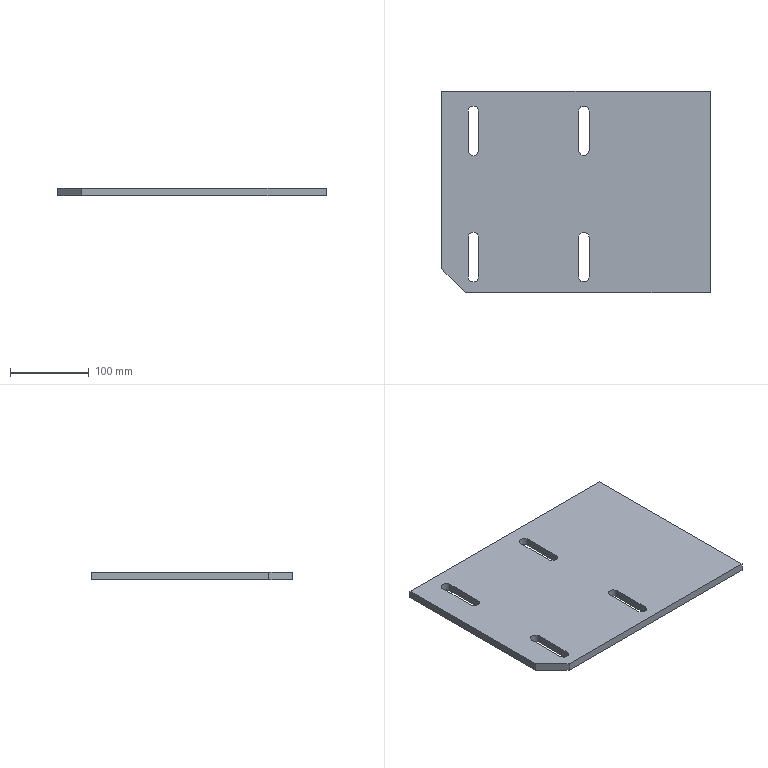Part | SolidWorks | features Extrusion 1 | 1 solid | 23 faces | box 340 x 255 x 10 mm | volume 831191 mm3 | plane 15 | cylinder 8 | commonest cylinder face diameters 13 x8
STEP:
#1=CARTESIAN_POINT('',(0.,-255.,0.));
#2=VERTEX_POINT('',#1);
#3=CARTESIAN_POINT('',(0.,0.,0.));
#4=VERTEX_POINT('',#3);
#5=CARTESIAN_POINT('',(0.,-255.,0.));
#6=DIRECTION('',(0.,1.,0.));
#7=VECTOR('',#6,1000.);
#8=LINE('',#5,#7);
#9=EDGE_CURVE('',#2,#4,#8,.T.);
#10=ORIENTED_EDGE('',*,*,#9,.F.);
#11=CARTESIAN_POINT('',(0.,-255.,-10.));
#12=VERTEX_POINT('',#11);
#13=CARTESIAN_POINT('',(0.,-255.,-10.));
#14=DIRECTION('',(0.,0.,1.));
#15=VECTOR('',#14,1000.);
#16=LINE('',#13,#15);
#17=EDGE_CURVE('',#12,#2,#16,.T.);
#18=ORIENTED_EDGE('',*,*,#17,.F.);
#19=CARTESIAN_POINT('',(0.,0.,-10.));
#20=VERTEX_POINT('',#19);
#21=CARTESIAN_POINT('',(0.,-255.,-10.));
#22=DIRECTION('',(0.,1.,0.));
#23=VECTOR('',#22,1000.);
#24=LINE('',#21,#23);
#25=EDGE_CURVE('',#12,#20,#24,.T.);
#26=ORIENTED_EDGE('',*,*,#25,.T.);
#27=CARTESIAN_POINT('',(0.,0.,-10.));
#28=DIRECTION('',(0.,0.,1.));
#29=VECTOR('',#28,1000.);
#30=LINE('',#27,#29);
#31=EDGE_CURVE('',#20,#4,#30,.T.);
#32=ORIENTED_EDGE('',*,*,#31,.T.);
#33=EDGE_LOOP('',(#10,#18,#26,#32));
#34=FACE_OUTER_BOUND('',#33,.T.);
#35=CARTESIAN_POINT('',(0.,-255.,-10.));
#36=DIRECTION('',(1.,0.,0.));
#37=DIRECTION('',(0.,1.,0.));
#38=AXIS2_PLACEMENT_3D('',#35,#36,#37);
#39=PLANE('',#38);
#40=ADVANCED_FACE('',(#34),#39,.T.);
#41=CARTESIAN_POINT('',(-310.,-255.,0.));
#42=VERTEX_POINT('',#41);
#43=CARTESIAN_POINT('',(-310.,-255.,0.));
#44=DIRECTION('',(1.,0.,0.));
#45=VECTOR('',#44,1000.);
#46=LINE('',#43,#45);
#47=EDGE_CURVE('',#42,#2,#46,.T.);
#48=ORIENTED_EDGE('',*,*,#47,.F.);
#49=CARTESIAN_POINT('',(-310.,-255.,-10.));
#50=VERTEX_POINT('',#49);
#51=CARTESIAN_POINT('',(-310.,-255.,-10.));
#52=DIRECTION('',(0.,0.,1.));
#53=VECTOR('',#52,1000.);
#54=LINE('',#51,#53);
#55=EDGE_CURVE('',#50,#42,#54,.T.);
#56=ORIENTED_EDGE('',*,*,#55,.F.);
#57=CARTESIAN_POINT('',(-310.,-255.,-10.));
#58=DIRECTION('',(1.,0.,0.));
#59=VECTOR('',#58,1000.);
#60=LINE('',#57,#59);
#61=EDGE_CURVE('',#50,#12,#60,.T.);
#62=ORIENTED_EDGE('',*,*,#61,.T.);
#63=ORIENTED_EDGE('',*,*,#17,.T.);
#64=EDGE_LOOP('',(#48,#56,#62,#63));
#65=FACE_OUTER_BOUND('',#64,.T.);
#66=CARTESIAN_POINT('',(-310.,-255.,-10.));
#67=DIRECTION('',(0.,-1.,0.));
#68=DIRECTION('',(0.,0.,-1.));
#69=AXIS2_PLACEMENT_3D('',#66,#67,#68);
#70=PLANE('',#69);
#71=ADVANCED_FACE('',(#65),#70,.T.);
#72=CARTESIAN_POINT('',(-340.,-225.,0.));
#73=VERTEX_POINT('',#72);
#74=CARTESIAN_POINT('',(-340.,-225.,0.));
#75=DIRECTION('',(0.7071,-0.7071,0.));
#76=VECTOR('',#75,1000.);
#77=LINE('',#74,#76);
#78=EDGE_CURVE('',#73,#42,#77,.T.);
#79=ORIENTED_EDGE('',*,*,#78,.F.);
#80=CARTESIAN_POINT('',(-340.,-225.,-10.));
#81=VERTEX_POINT('',#80);
#82=CARTESIAN_POINT('',(-340.,-225.,-10.));
#83=DIRECTION('',(0.,0.,1.));
#84=VECTOR('',#83,1000.);
#85=LINE('',#82,#84);
#86=EDGE_CURVE('',#81,#73,#85,.T.);
#87=ORIENTED_EDGE('',*,*,#86,.F.);
#88=CARTESIAN_POINT('',(-340.,-225.,-10.));
#89=DIRECTION('',(0.7071,-0.7071,0.));
#90=VECTOR('',#89,1000.);
#91=LINE('',#88,#90);
#92=EDGE_CURVE('',#81,#50,#91,.T.);
#93=ORIENTED_EDGE('',*,*,#92,.T.);
#94=ORIENTED_EDGE('',*,*,#55,.T.);
#95=EDGE_LOOP('',(#79,#87,#93,#94));
#96=FACE_OUTER_BOUND('',#95,.T.);
#97=CARTESIAN_POINT('',(-340.,-225.,-10.));
#98=DIRECTION('',(-0.7071,-0.7071,0.));
#99=DIRECTION('',(0.7071,-0.7071,0.));
#100=AXIS2_PLACEMENT_3D('',#97,#98,#99);
#101=PLANE('',#100);
#102=ADVANCED_FACE('',(#96),#101,.T.);
#103=CARTESIAN_POINT('',(-340.,0.,0.));
#104=VERTEX_POINT('',#103);
#105=CARTESIAN_POINT('',(-340.,0.,0.));
#106=DIRECTION('',(0.,-1.,0.));
#107=VECTOR('',#106,1000.);
#108=LINE('',#105,#107);
#109=EDGE_CURVE('',#104,#73,#108,.T.);
#110=ORIENTED_EDGE('',*,*,#109,.F.);
#111=CARTESIAN_POINT('',(-340.,0.,-10.));
#112=VERTEX_POINT('',#111);
#113=CARTESIAN_POINT('',(-340.,0.,-10.));
#114=DIRECTION('',(0.,0.,1.));
#115=VECTOR('',#114,1000.);
#116=LINE('',#113,#115);
#117=EDGE_CURVE('',#112,#104,#116,.T.);
#118=ORIENTED_EDGE('',*,*,#117,.F.);
#119=CARTESIAN_POINT('',(-340.,0.,-10.));
#120=DIRECTION('',(0.,-1.,0.));
#121=VECTOR('',#120,1000.);
#122=LINE('',#119,#121);
#123=EDGE_CURVE('',#112,#81,#122,.T.);
#124=ORIENTED_EDGE('',*,*,#123,.T.);
#125=ORIENTED_EDGE('',*,*,#86,.T.);
#126=EDGE_LOOP('',(#110,#118,#124,#125));
#127=FACE_OUTER_BOUND('',#126,.T.);
#128=CARTESIAN_POINT('',(-340.,0.,-10.));
#129=DIRECTION('',(-1.,0.,0.));
#130=DIRECTION('',(0.,-1.,0.));
#131=AXIS2_PLACEMENT_3D('',#128,#129,#130);
#132=PLANE('',#131);
#133=ADVANCED_FACE('',(#127),#132,.T.);
#134=CARTESIAN_POINT('',(0.,0.,0.));
#135=DIRECTION('',(-1.,0.,0.));
#136=VECTOR('',#135,1000.);
#137=LINE('',#134,#136);
#138=EDGE_CURVE('',#4,#104,#137,.T.);
#139=ORIENTED_EDGE('',*,*,#138,.F.);
#140=ORIENTED_EDGE('',*,*,#31,.F.);
#141=CARTESIAN_POINT('',(0.,0.,-10.));
#142=DIRECTION('',(-1.,0.,0.));
#143=VECTOR('',#142,1000.);
#144=LINE('',#141,#143);
#145=EDGE_CURVE('',#20,#112,#144,.T.);
#146=ORIENTED_EDGE('',*,*,#145,.T.);
#147=ORIENTED_EDGE('',*,*,#117,.T.);
#148=EDGE_LOOP('',(#139,#140,#146,#147));
#149=FACE_OUTER_BOUND('',#148,.T.);
#150=CARTESIAN_POINT('',(0.,0.,-10.));
#151=DIRECTION('',(0.,1.,0.));
#152=DIRECTION('',(-1.,0.,0.));
#153=AXIS2_PLACEMENT_3D('',#150,#151,#152);
#154=PLANE('',#153);
#155=ADVANCED_FACE('',(#149),#154,.T.);
#156=CARTESIAN_POINT('',(-153.5,-235.,-10.));
#157=VERTEX_POINT('',#156);
#158=CARTESIAN_POINT('',(-153.5,-185.,-10.));
#159=VERTEX_POINT('',#158);
#160=CARTESIAN_POINT('',(-153.5,-185.,-10.));
#161=DIRECTION('',(0.,1.,0.));
#162=VECTOR('',#161,1000.);
#163=LINE('',#160,#162);
#164=EDGE_CURVE('',#157,#159,#163,.T.);
#165=ORIENTED_EDGE('',*,*,#164,.T.);
#166=CARTESIAN_POINT('',(-166.5,-185.,-10.));
#167=VERTEX_POINT('',#166);
#168=CARTESIAN_POINT('',(-160.,-185.,-10.));
#169=DIRECTION('',(0.,0.,1.));
#170=DIRECTION('',(1.,0.,0.));
#171=AXIS2_PLACEMENT_3D('',#168,#169,#170);
#172=CIRCLE('',#171,6.5);
#173=EDGE_CURVE('',#159,#167,#172,.T.);
#174=ORIENTED_EDGE('',*,*,#173,.T.);
#175=CARTESIAN_POINT('',(-166.5,-235.,-10.));
#176=VERTEX_POINT('',#175);
#177=CARTESIAN_POINT('',(-166.5,-185.,-10.));
#178=DIRECTION('',(0.,-1.,0.));
#179=VECTOR('',#178,1000.);
#180=LINE('',#177,#179);
#181=EDGE_CURVE('',#167,#176,#180,.T.);
#182=ORIENTED_EDGE('',*,*,#181,.T.);
#183=CARTESIAN_POINT('',(-160.,-235.,-10.));
#184=DIRECTION('',(0.,0.,1.));
#185=DIRECTION('',(1.,0.,0.));
#186=AXIS2_PLACEMENT_3D('',#183,#184,#185);
#187=CIRCLE('',#186,6.5);
#188=EDGE_CURVE('',#176,#157,#187,.T.);
#189=ORIENTED_EDGE('',*,*,#188,.T.);
#190=EDGE_LOOP('',(#165,#174,#182,#189));
#191=FACE_BOUND('',#190,.T.);
#192=CARTESIAN_POINT('',(-293.5,-235.,-10.));
#193=VERTEX_POINT('',#192);
#194=CARTESIAN_POINT('',(-293.5,-185.,-10.));
#195=VERTEX_POINT('',#194);
#196=CARTESIAN_POINT('',(-293.5,-185.,-10.));
#197=DIRECTION('',(0.,1.,0.));
#198=VECTOR('',#197,1000.);
#199=LINE('',#196,#198);
#200=EDGE_CURVE('',#193,#195,#199,.T.);
#201=ORIENTED_EDGE('',*,*,#200,.T.);
#202=CARTESIAN_POINT('',(-306.5,-185.,-10.));
#203=VERTEX_POINT('',#202);
#204=CARTESIAN_POINT('',(-300.,-185.,-10.));
#205=DIRECTION('',(0.,0.,1.));
#206=DIRECTION('',(1.,0.,0.));
#207=AXIS2_PLACEMENT_3D('',#204,#205,#206);
#208=CIRCLE('',#207,6.5);
#209=EDGE_CURVE('',#195,#203,#208,.T.);
#210=ORIENTED_EDGE('',*,*,#209,.T.);
#211=CARTESIAN_POINT('',(-306.5,-235.,-10.));
#212=VERTEX_POINT('',#211);
#213=CARTESIAN_POINT('',(-306.5,-185.,-10.));
#214=DIRECTION('',(0.,-1.,0.));
#215=VECTOR('',#214,1000.);
#216=LINE('',#213,#215);
#217=EDGE_CURVE('',#203,#212,#216,.T.);
#218=ORIENTED_EDGE('',*,*,#217,.T.);
#219=CARTESIAN_POINT('',(-300.,-235.,-10.));
#220=DIRECTION('',(0.,0.,1.));
#221=DIRECTION('',(1.,0.,0.));
#222=AXIS2_PLACEMENT_3D('',#219,#220,#221);
#223=CIRCLE('',#222,6.5);
#224=EDGE_CURVE('',#212,#193,#223,.T.);
#225=ORIENTED_EDGE('',*,*,#224,.T.);
#226=EDGE_LOOP('',(#201,#210,#218,#225));
#227=FACE_BOUND('',#226,.T.);
#228=CARTESIAN_POINT('',(-153.5,-75.,-10.));
#229=VERTEX_POINT('',#228);
#230=CARTESIAN_POINT('',(-153.5,-25.,-10.));
#231=VERTEX_POINT('',#230);
#232=CARTESIAN_POINT('',(-153.5,-25.,-10.));
#233=DIRECTION('',(0.,1.,0.));
#234=VECTOR('',#233,1000.);
#235=LINE('',#232,#234);
#236=EDGE_CURVE('',#229,#231,#235,.T.);
#237=ORIENTED_EDGE('',*,*,#236,.T.);
#238=CARTESIAN_POINT('',(-166.5,-25.,-10.));
#239=VERTEX_POINT('',#238);
#240=CARTESIAN_POINT('',(-160.,-25.,-10.));
#241=DIRECTION('',(0.,0.,1.));
#242=DIRECTION('',(1.,0.,0.));
#243=AXIS2_PLACEMENT_3D('',#240,#241,#242);
#244=CIRCLE('',#243,6.5);
#245=EDGE_CURVE('',#231,#239,#244,.T.);
#246=ORIENTED_EDGE('',*,*,#245,.T.);
#247=CARTESIAN_POINT('',(-166.5,-75.,-10.));
#248=VERTEX_POINT('',#247);
#249=CARTESIAN_POINT('',(-166.5,-25.,-10.));
#250=DIRECTION('',(0.,-1.,0.));
#251=VECTOR('',#250,1000.);
#252=LINE('',#249,#251);
#253=EDGE_CURVE('',#239,#248,#252,.T.);
#254=ORIENTED_EDGE('',*,*,#253,.T.);
#255=CARTESIAN_POINT('',(-160.,-75.,-10.));
#256=DIRECTION('',(0.,0.,1.));
#257=DIRECTION('',(1.,0.,0.));
#258=AXIS2_PLACEMENT_3D('',#255,#256,#257);
#259=CIRCLE('',#258,6.5);
#260=EDGE_CURVE('',#248,#229,#259,.T.);
#261=ORIENTED_EDGE('',*,*,#260,.T.);
#262=EDGE_LOOP('',(#237,#246,#254,#261));
#263=FACE_BOUND('',#262,.T.);
#264=CARTESIAN_POINT('',(-293.5,-75.,-10.));
#265=VERTEX_POINT('',#264);
#266=CARTESIAN_POINT('',(-293.5,-25.,-10.));
#267=VERTEX_POINT('',#266);
#268=CARTESIAN_POINT('',(-293.5,-25.,-10.));
#269=DIRECTION('',(0.,1.,0.));
#270=VECTOR('',#269,1000.);
#271=LINE('',#268,#270);
#272=EDGE_CURVE('',#265,#267,#271,.T.);
#273=ORIENTED_EDGE('',*,*,#272,.T.);
#274=CARTESIAN_POINT('',(-306.5,-25.,-10.));
#275=VERTEX_POINT('',#274);
#276=CARTESIAN_POINT('',(-300.,-25.,-10.));
#277=DIRECTION('',(0.,0.,1.));
#278=DIRECTION('',(1.,0.,0.));
#279=AXIS2_PLACEMENT_3D('',#276,#277,#278);
#280=CIRCLE('',#279,6.5);
#281=EDGE_CURVE('',#267,#275,#280,.T.);
#282=ORIENTED_EDGE('',*,*,#281,.T.);
#283=CARTESIAN_POINT('',(-306.5,-75.,-10.));
#284=VERTEX_POINT('',#283);
#285=CARTESIAN_POINT('',(-306.5,-25.,-10.));
#286=DIRECTION('',(0.,-1.,0.));
#287=VECTOR('',#286,1000.);
#288=LINE('',#285,#287);
#289=EDGE_CURVE('',#275,#284,#288,.T.);
#290=ORIENTED_EDGE('',*,*,#289,.T.);
#291=CARTESIAN_POINT('',(-300.,-75.,-10.));
#292=DIRECTION('',(0.,0.,1.));
#293=DIRECTION('',(1.,0.,0.));
#294=AXIS2_PLACEMENT_3D('',#291,#292,#293);
#295=CIRCLE('',#294,6.5);
#296=EDGE_CURVE('',#284,#265,#295,.T.);
#297=ORIENTED_EDGE('',*,*,#296,.T.);
#298=EDGE_LOOP('',(#273,#282,#290,#297));
#299=FACE_BOUND('',#298,.T.);
#300=ORIENTED_EDGE('',*,*,#25,.F.);
#301=ORIENTED_EDGE('',*,*,#61,.F.);
#302=ORIENTED_EDGE('',*,*,#92,.F.);
#303=ORIENTED_EDGE('',*,*,#123,.F.);
#304=ORIENTED_EDGE('',*,*,#145,.F.);
#305=EDGE_LOOP('',(#300,#301,#302,#303,#304));
#306=FACE_OUTER_BOUND('',#305,.T.);
#307=CARTESIAN_POINT('',(0.,0.,-10.));
#308=DIRECTION('',(0.,0.,1.));
#309=DIRECTION('',(1.,0.,0.));
#310=AXIS2_PLACEMENT_3D('',#307,#308,#309);
#311=PLANE('',#310);
#312=ADVANCED_FACE('',(#191,#227,#263,#299,#306),#311,.F.);
#313=CARTESIAN_POINT('',(-153.5,-185.,0.));
#314=VERTEX_POINT('',#313);
#315=CARTESIAN_POINT('',(-166.5,-185.,0.));
#316=VERTEX_POINT('',#315);
#317=CARTESIAN_POINT('',(-160.,-185.,0.));
#318=DIRECTION('',(0.,0.,1.));
#319=DIRECTION('',(1.,0.,0.));
#320=AXIS2_PLACEMENT_3D('',#317,#318,#319);
#321=CIRCLE('',#320,6.5);
#322=EDGE_CURVE('',#314,#316,#321,.T.);
#323=ORIENTED_EDGE('',*,*,#322,.F.);
#324=CARTESIAN_POINT('',(-153.5,-235.,0.));
#325=VERTEX_POINT('',#324);
#326=CARTESIAN_POINT('',(-153.5,-185.,0.));
#327=DIRECTION('',(0.,1.,0.));
#328=VECTOR('',#327,1000.);
#329=LINE('',#326,#328);
#330=EDGE_CURVE('',#325,#314,#329,.T.);
#331=ORIENTED_EDGE('',*,*,#330,.F.);
#332=CARTESIAN_POINT('',(-166.5,-235.,0.));
#333=VERTEX_POINT('',#332);
#334=CARTESIAN_POINT('',(-160.,-235.,0.));
#335=DIRECTION('',(0.,0.,1.));
#336=DIRECTION('',(1.,0.,0.));
#337=AXIS2_PLACEMENT_3D('',#334,#335,#336);
#338=CIRCLE('',#337,6.5);
#339=EDGE_CURVE('',#333,#325,#338,.T.);
#340=ORIENTED_EDGE('',*,*,#339,.F.);
#341=CARTESIAN_POINT('',(-166.5,-185.,0.));
#342=DIRECTION('',(0.,-1.,0.));
#343=VECTOR('',#342,1000.);
#344=LINE('',#341,#343);
#345=EDGE_CURVE('',#316,#333,#344,.T.);
#346=ORIENTED_EDGE('',*,*,#345,.F.);
#347=EDGE_LOOP('',(#323,#331,#340,#346));
#348=FACE_BOUND('',#347,.T.);
#349=CARTESIAN_POINT('',(-293.5,-185.,0.));
#350=VERTEX_POINT('',#349);
#351=CARTESIAN_POINT('',(-306.5,-185.,0.));
#352=VERTEX_POINT('',#351);
#353=CARTESIAN_POINT('',(-300.,-185.,0.));
#354=DIRECTION('',(0.,0.,1.));
#355=DIRECTION('',(1.,0.,0.));
#356=AXIS2_PLACEMENT_3D('',#353,#354,#355);
#357=CIRCLE('',#356,6.5);
#358=EDGE_CURVE('',#350,#352,#357,.T.);
#359=ORIENTED_EDGE('',*,*,#358,.F.);
#360=CARTESIAN_POINT('',(-293.5,-235.,0.));
#361=VERTEX_POINT('',#360);
#362=CARTESIAN_POINT('',(-293.5,-185.,0.));
#363=DIRECTION('',(0.,1.,0.));
#364=VECTOR('',#363,1000.);
#365=LINE('',#362,#364);
#366=EDGE_CURVE('',#361,#350,#365,.T.);
#367=ORIENTED_EDGE('',*,*,#366,.F.);
#368=CARTESIAN_POINT('',(-306.5,-235.,0.));
#369=VERTEX_POINT('',#368);
#370=CARTESIAN_POINT('',(-300.,-235.,0.));
#371=DIRECTION('',(0.,0.,1.));
#372=DIRECTION('',(1.,0.,0.));
#373=AXIS2_PLACEMENT_3D('',#370,#371,#372);
#374=CIRCLE('',#373,6.5);
#375=EDGE_CURVE('',#369,#361,#374,.T.);
#376=ORIENTED_EDGE('',*,*,#375,.F.);
#377=CARTESIAN_POINT('',(-306.5,-185.,0.));
#378=DIRECTION('',(0.,-1.,0.));
#379=VECTOR('',#378,1000.);
#380=LINE('',#377,#379);
#381=EDGE_CURVE('',#352,#369,#380,.T.);
#382=ORIENTED_EDGE('',*,*,#381,.F.);
#383=EDGE_LOOP('',(#359,#367,#376,#382));
#384=FACE_BOUND('',#383,.T.);
#385=CARTESIAN_POINT('',(-153.5,-25.,0.));
#386=VERTEX_POINT('',#385);
#387=CARTESIAN_POINT('',(-166.5,-25.,0.));
#388=VERTEX_POINT('',#387);
#389=CARTESIAN_POINT('',(-160.,-25.,0.));
#390=DIRECTION('',(0.,0.,1.));
#391=DIRECTION('',(1.,0.,0.));
#392=AXIS2_PLACEMENT_3D('',#389,#390,#391);
#393=CIRCLE('',#392,6.5);
#394=EDGE_CURVE('',#386,#388,#393,.T.);
#395=ORIENTED_EDGE('',*,*,#394,.F.);
#396=CARTESIAN_POINT('',(-153.5,-75.,0.));
#397=VERTEX_POINT('',#396);
#398=CARTESIAN_POINT('',(-153.5,-25.,0.));
#399=DIRECTION('',(0.,1.,0.));
#400=VECTOR('',#399,1000.);
#401=LINE('',#398,#400);
#402=EDGE_CURVE('',#397,#386,#401,.T.);
#403=ORIENTED_EDGE('',*,*,#402,.F.);
#404=CARTESIAN_POINT('',(-166.5,-75.,0.));
#405=VERTEX_POINT('',#404);
#406=CARTESIAN_POINT('',(-160.,-75.,0.));
#407=DIRECTION('',(0.,0.,1.));
#408=DIRECTION('',(1.,0.,0.));
#409=AXIS2_PLACEMENT_3D('',#406,#407,#408);
#410=CIRCLE('',#409,6.5);
#411=EDGE_CURVE('',#405,#397,#410,.T.);
#412=ORIENTED_EDGE('',*,*,#411,.F.);
#413=CARTESIAN_POINT('',(-166.5,-25.,0.));
#414=DIRECTION('',(0.,-1.,0.));
#415=VECTOR('',#414,1000.);
#416=LINE('',#413,#415);
#417=EDGE_CURVE('',#388,#405,#416,.T.);
#418=ORIENTED_EDGE('',*,*,#417,.F.);
#419=EDGE_LOOP('',(#395,#403,#412,#418));
#420=FACE_BOUND('',#419,.T.);
#421=CARTESIAN_POINT('',(-293.5,-25.,0.));
#422=VERTEX_POINT('',#421);
#423=CARTESIAN_POINT('',(-306.5,-25.,0.));
#424=VERTEX_POINT('',#423);
#425=CARTESIAN_POINT('',(-300.,-25.,0.));
#426=DIRECTION('',(0.,0.,1.));
#427=DIRECTION('',(1.,0.,0.));
#428=AXIS2_PLACEMENT_3D('',#425,#426,#427);
#429=CIRCLE('',#428,6.5);
#430=EDGE_CURVE('',#422,#424,#429,.T.);
#431=ORIENTED_EDGE('',*,*,#430,.F.);
#432=CARTESIAN_POINT('',(-293.5,-75.,0.));
#433=VERTEX_POINT('',#432);
#434=CARTESIAN_POINT('',(-293.5,-25.,0.));
#435=DIRECTION('',(0.,1.,0.));
#436=VECTOR('',#435,1000.);
#437=LINE('',#434,#436);
#438=EDGE_CURVE('',#433,#422,#437,.T.);
#439=ORIENTED_EDGE('',*,*,#438,.F.);
#440=CARTESIAN_POINT('',(-306.5,-75.,0.));
#441=VERTEX_POINT('',#440);
#442=CARTESIAN_POINT('',(-300.,-75.,0.));
#443=DIRECTION('',(0.,0.,1.));
#444=DIRECTION('',(1.,0.,0.));
#445=AXIS2_PLACEMENT_3D('',#442,#443,#444);
#446=CIRCLE('',#445,6.5);
#447=EDGE_CURVE('',#441,#433,#446,.T.);
#448=ORIENTED_EDGE('',*,*,#447,.F.);
#449=CARTESIAN_POINT('',(-306.5,-25.,0.));
#450=DIRECTION('',(0.,-1.,0.));
#451=VECTOR('',#450,1000.);
#452=LINE('',#449,#451);
#453=EDGE_CURVE('',#424,#441,#452,.T.);
#454=ORIENTED_EDGE('',*,*,#453,.F.);
#455=EDGE_LOOP('',(#431,#439,#448,#454));
#456=FACE_BOUND('',#455,.T.);
#457=ORIENTED_EDGE('',*,*,#9,.T.);
#458=ORIENTED_EDGE('',*,*,#138,.T.);
#459=ORIENTED_EDGE('',*,*,#109,.T.);
#460=ORIENTED_EDGE('',*,*,#78,.T.);
#461=ORIENTED_EDGE('',*,*,#47,.T.);
#462=EDGE_LOOP('',(#457,#458,#459,#460,#461));
#463=FACE_OUTER_BOUND('',#462,.T.);
#464=CARTESIAN_POINT('',(0.,0.,0.));
#465=DIRECTION('',(0.,0.,1.));
#466=DIRECTION('',(1.,0.,0.));
#467=AXIS2_PLACEMENT_3D('',#464,#465,#466);
#468=PLANE('',#467);
#469=ADVANCED_FACE('',(#348,#384,#420,#456,#463),#468,.T.);
#470=ORIENTED_EDGE('',*,*,#430,.T.);
#471=CARTESIAN_POINT('',(-306.5,-25.,-10.));
#472=DIRECTION('',(0.,0.,1.));
#473=VECTOR('',#472,1000.);
#474=LINE('',#471,#473);
#475=EDGE_CURVE('',#275,#424,#474,.T.);
#476=ORIENTED_EDGE('',*,*,#475,.F.);
#477=ORIENTED_EDGE('',*,*,#281,.F.);
#478=CARTESIAN_POINT('',(-293.5,-25.,-10.));
#479=DIRECTION('',(0.,0.,1.));
#480=VECTOR('',#479,1000.);
#481=LINE('',#478,#480);
#482=EDGE_CURVE('',#267,#422,#481,.T.);
#483=ORIENTED_EDGE('',*,*,#482,.T.);
#484=EDGE_LOOP('',(#470,#476,#477,#483));
#485=FACE_OUTER_BOUND('',#484,.T.);
#486=CARTESIAN_POINT('',(-300.,-25.,-10.));
#487=DIRECTION('',(0.,0.,1.));
#488=DIRECTION('',(1.,0.,0.));
#489=AXIS2_PLACEMENT_3D('',#486,#487,#488);
#490=CYLINDRICAL_SURFACE('',#489,6.5);
#491=ADVANCED_FACE('',(#485),#490,.F.);
#492=ORIENTED_EDGE('',*,*,#438,.T.);
#493=ORIENTED_EDGE('',*,*,#482,.F.);
#494=ORIENTED_EDGE('',*,*,#272,.F.);
#495=CARTESIAN_POINT('',(-293.5,-75.,-10.));
#496=DIRECTION('',(0.,0.,1.));
#497=VECTOR('',#496,1000.);
#498=LINE('',#495,#497);
#499=EDGE_CURVE('',#265,#433,#498,.T.);
#500=ORIENTED_EDGE('',*,*,#499,.T.);
#501=EDGE_LOOP('',(#492,#493,#494,#500));
#502=FACE_OUTER_BOUND('',#501,.T.);
#503=CARTESIAN_POINT('',(-293.5,-25.,-10.));
#504=DIRECTION('',(1.,0.,0.));
#505=DIRECTION('',(0.,0.,-1.));
#506=AXIS2_PLACEMENT_3D('',#503,#504,#505);
#507=PLANE('',#506);
#508=ADVANCED_FACE('',(#502),#507,.F.);
#509=ORIENTED_EDGE('',*,*,#447,.T.);
#510=ORIENTED_EDGE('',*,*,#499,.F.);
#511=ORIENTED_EDGE('',*,*,#296,.F.);
#512=CARTESIAN_POINT('',(-306.5,-75.,-10.));
#513=DIRECTION('',(0.,0.,1.));
#514=VECTOR('',#513,1000.);
#515=LINE('',#512,#514);
#516=EDGE_CURVE('',#284,#441,#515,.T.);
#517=ORIENTED_EDGE('',*,*,#516,.T.);
#518=EDGE_LOOP('',(#509,#510,#511,#517));
#519=FACE_OUTER_BOUND('',#518,.T.);
#520=CARTESIAN_POINT('',(-300.,-75.,-10.));
#521=DIRECTION('',(0.,0.,1.));
#522=DIRECTION('',(1.,0.,0.));
#523=AXIS2_PLACEMENT_3D('',#520,#521,#522);
#524=CYLINDRICAL_SURFACE('',#523,6.5);
#525=ADVANCED_FACE('',(#519),#524,.F.);
#526=ORIENTED_EDGE('',*,*,#453,.T.);
#527=ORIENTED_EDGE('',*,*,#516,.F.);
#528=ORIENTED_EDGE('',*,*,#289,.F.);
#529=ORIENTED_EDGE('',*,*,#475,.T.);
#530=EDGE_LOOP('',(#526,#527,#528,#529));
#531=FACE_OUTER_BOUND('',#530,.T.);
#532=CARTESIAN_POINT('',(-306.5,-25.,-10.));
#533=DIRECTION('',(-1.,0.,0.));
#534=DIRECTION('',(0.,0.,1.));
#535=AXIS2_PLACEMENT_3D('',#532,#533,#534);
#536=PLANE('',#535);
#537=ADVANCED_FACE('',(#531),#536,.F.);
#538=ORIENTED_EDGE('',*,*,#394,.T.);
#539=CARTESIAN_POINT('',(-166.5,-25.,-10.));
#540=DIRECTION('',(0.,0.,1.));
#541=VECTOR('',#540,1000.);
#542=LINE('',#539,#541);
#543=EDGE_CURVE('',#239,#388,#542,.T.);
#544=ORIENTED_EDGE('',*,*,#543,.F.);
#545=ORIENTED_EDGE('',*,*,#245,.F.);
#546=CARTESIAN_POINT('',(-153.5,-25.,-10.));
#547=DIRECTION('',(0.,0.,1.));
#548=VECTOR('',#547,1000.);
#549=LINE('',#546,#548);
#550=EDGE_CURVE('',#231,#386,#549,.T.);
#551=ORIENTED_EDGE('',*,*,#550,.T.);
#552=EDGE_LOOP('',(#538,#544,#545,#551));
#553=FACE_OUTER_BOUND('',#552,.T.);
#554=CARTESIAN_POINT('',(-160.,-25.,-10.));
#555=DIRECTION('',(0.,0.,1.));
#556=DIRECTION('',(1.,0.,0.));
#557=AXIS2_PLACEMENT_3D('',#554,#555,#556);
#558=CYLINDRICAL_SURFACE('',#557,6.5);
#559=ADVANCED_FACE('',(#553),#558,.F.);
#560=ORIENTED_EDGE('',*,*,#402,.T.);
#561=ORIENTED_EDGE('',*,*,#550,.F.);
#562=ORIENTED_EDGE('',*,*,#236,.F.);
#563=CARTESIAN_POINT('',(-153.5,-75.,-10.));
#564=DIRECTION('',(0.,0.,1.));
#565=VECTOR('',#564,1000.);
#566=LINE('',#563,#565);
#567=EDGE_CURVE('',#229,#397,#566,.T.);
#568=ORIENTED_EDGE('',*,*,#567,.T.);
#569=EDGE_LOOP('',(#560,#561,#562,#568));
#570=FACE_OUTER_BOUND('',#569,.T.);
#571=CARTESIAN_POINT('',(-153.5,-25.,-10.));
#572=DIRECTION('',(1.,0.,0.));
#573=DIRECTION('',(0.,0.,-1.));
#574=AXIS2_PLACEMENT_3D('',#571,#572,#573);
#575=PLANE('',#574);
#576=ADVANCED_FACE('',(#570),#575,.F.);
#577=ORIENTED_EDGE('',*,*,#411,.T.);
#578=ORIENTED_EDGE('',*,*,#567,.F.);
#579=ORIENTED_EDGE('',*,*,#260,.F.);
#580=CARTESIAN_POINT('',(-166.5,-75.,-10.));
#581=DIRECTION('',(0.,0.,1.));
#582=VECTOR('',#581,1000.);
#583=LINE('',#580,#582);
#584=EDGE_CURVE('',#248,#405,#583,.T.);
#585=ORIENTED_EDGE('',*,*,#584,.T.);
#586=EDGE_LOOP('',(#577,#578,#579,#585));
#587=FACE_OUTER_BOUND('',#586,.T.);
#588=CARTESIAN_POINT('',(-160.,-75.,-10.));
#589=DIRECTION('',(0.,0.,1.));
#590=DIRECTION('',(1.,0.,0.));
#591=AXIS2_PLACEMENT_3D('',#588,#589,#590);
#592=CYLINDRICAL_SURFACE('',#591,6.5);
#593=ADVANCED_FACE('',(#587),#592,.F.);
#594=ORIENTED_EDGE('',*,*,#417,.T.);
#595=ORIENTED_EDGE('',*,*,#584,.F.);
#596=ORIENTED_EDGE('',*,*,#253,.F.);
#597=ORIENTED_EDGE('',*,*,#543,.T.);
#598=EDGE_LOOP('',(#594,#595,#596,#597));
#599=FACE_OUTER_BOUND('',#598,.T.);
#600=CARTESIAN_POINT('',(-166.5,-25.,-10.));
#601=DIRECTION('',(-1.,0.,0.));
#602=DIRECTION('',(0.,0.,1.));
#603=AXIS2_PLACEMENT_3D('',#600,#601,#602);
#604=PLANE('',#603);
#605=ADVANCED_FACE('',(#599),#604,.F.);
#606=ORIENTED_EDGE('',*,*,#358,.T.);
#607=CARTESIAN_POINT('',(-306.5,-185.,-10.));
#608=DIRECTION('',(0.,0.,1.));
#609=VECTOR('',#608,1000.);
#610=LINE('',#607,#609);
#611=EDGE_CURVE('',#203,#352,#610,.T.);
#612=ORIENTED_EDGE('',*,*,#611,.F.);
#613=ORIENTED_EDGE('',*,*,#209,.F.);
#614=CARTESIAN_POINT('',(-293.5,-185.,-10.));
#615=DIRECTION('',(0.,0.,1.));
#616=VECTOR('',#615,1000.);
#617=LINE('',#614,#616);
#618=EDGE_CURVE('',#195,#350,#617,.T.);
#619=ORIENTED_EDGE('',*,*,#618,.T.);
#620=EDGE_LOOP('',(#606,#612,#613,#619));
#621=FACE_OUTER_BOUND('',#620,.T.);
#622=CARTESIAN_POINT('',(-300.,-185.,-10.));
#623=DIRECTION('',(0.,0.,1.));
#624=DIRECTION('',(1.,0.,0.));
#625=AXIS2_PLACEMENT_3D('',#622,#623,#624);
#626=CYLINDRICAL_SURFACE('',#625,6.5);
#627=ADVANCED_FACE('',(#621),#626,.F.);
#628=ORIENTED_EDGE('',*,*,#366,.T.);
#629=ORIENTED_EDGE('',*,*,#618,.F.);
#630=ORIENTED_EDGE('',*,*,#200,.F.);
#631=CARTESIAN_POINT('',(-293.5,-235.,-10.));
#632=DIRECTION('',(0.,0.,1.));
#633=VECTOR('',#632,1000.);
#634=LINE('',#631,#633);
#635=EDGE_CURVE('',#193,#361,#634,.T.);
#636=ORIENTED_EDGE('',*,*,#635,.T.);
#637=EDGE_LOOP('',(#628,#629,#630,#636));
#638=FACE_OUTER_BOUND('',#637,.T.);
#639=CARTESIAN_POINT('',(-293.5,-185.,-10.));
#640=DIRECTION('',(1.,0.,0.));
#641=DIRECTION('',(0.,0.,-1.));
#642=AXIS2_PLACEMENT_3D('',#639,#640,#641);
#643=PLANE('',#642);
#644=ADVANCED_FACE('',(#638),#643,.F.);
#645=ORIENTED_EDGE('',*,*,#375,.T.);
#646=ORIENTED_EDGE('',*,*,#635,.F.);
#647=ORIENTED_EDGE('',*,*,#224,.F.);
#648=CARTESIAN_POINT('',(-306.5,-235.,-10.));
#649=DIRECTION('',(0.,0.,1.));
#650=VECTOR('',#649,1000.);
#651=LINE('',#648,#650);
#652=EDGE_CURVE('',#212,#369,#651,.T.);
#653=ORIENTED_EDGE('',*,*,#652,.T.);
#654=EDGE_LOOP('',(#645,#646,#647,#653));
#655=FACE_OUTER_BOUND('',#654,.T.);
#656=CARTESIAN_POINT('',(-300.,-235.,-10.));
#657=DIRECTION('',(0.,0.,1.));
#658=DIRECTION('',(1.,0.,0.));
#659=AXIS2_PLACEMENT_3D('',#656,#657,#658);
#660=CYLINDRICAL_SURFACE('',#659,6.5);
#661=ADVANCED_FACE('',(#655),#660,.F.);
#662=ORIENTED_EDGE('',*,*,#381,.T.);
#663=ORIENTED_EDGE('',*,*,#652,.F.);
#664=ORIENTED_EDGE('',*,*,#217,.F.);
#665=ORIENTED_EDGE('',*,*,#611,.T.);
#666=EDGE_LOOP('',(#662,#663,#664,#665));
#667=FACE_OUTER_BOUND('',#666,.T.);
#668=CARTESIAN_POINT('',(-306.5,-185.,-10.));
#669=DIRECTION('',(-1.,0.,0.));
#670=DIRECTION('',(0.,0.,1.));
#671=AXIS2_PLACEMENT_3D('',#668,#669,#670);
#672=PLANE('',#671);
#673=ADVANCED_FACE('',(#667),#672,.F.);
#674=ORIENTED_EDGE('',*,*,#322,.T.);
#675=CARTESIAN_POINT('',(-166.5,-185.,-10.));
#676=DIRECTION('',(0.,0.,1.));
#677=VECTOR('',#676,1000.);
#678=LINE('',#675,#677);
#679=EDGE_CURVE('',#167,#316,#678,.T.);
#680=ORIENTED_EDGE('',*,*,#679,.F.);
#681=ORIENTED_EDGE('',*,*,#173,.F.);
#682=CARTESIAN_POINT('',(-153.5,-185.,-10.));
#683=DIRECTION('',(0.,0.,1.));
#684=VECTOR('',#683,1000.);
#685=LINE('',#682,#684);
#686=EDGE_CURVE('',#159,#314,#685,.T.);
#687=ORIENTED_EDGE('',*,*,#686,.T.);
#688=EDGE_LOOP('',(#674,#680,#681,#687));
#689=FACE_OUTER_BOUND('',#688,.T.);
#690=CARTESIAN_POINT('',(-160.,-185.,-10.));
#691=DIRECTION('',(0.,0.,1.));
#692=DIRECTION('',(1.,0.,0.));
#693=AXIS2_PLACEMENT_3D('',#690,#691,#692);
#694=CYLINDRICAL_SURFACE('',#693,6.5);
#695=ADVANCED_FACE('',(#689),#694,.F.);
#696=ORIENTED_EDGE('',*,*,#330,.T.);
#697=ORIENTED_EDGE('',*,*,#686,.F.);
#698=ORIENTED_EDGE('',*,*,#164,.F.);
#699=CARTESIAN_POINT('',(-153.5,-235.,-10.));
#700=DIRECTION('',(0.,0.,1.));
#701=VECTOR('',#700,1000.);
#702=LINE('',#699,#701);
#703=EDGE_CURVE('',#157,#325,#702,.T.);
#704=ORIENTED_EDGE('',*,*,#703,.T.);
#705=EDGE_LOOP('',(#696,#697,#698,#704));
#706=FACE_OUTER_BOUND('',#705,.T.);
#707=CARTESIAN_POINT('',(-153.5,-185.,-10.));
#708=DIRECTION('',(1.,0.,0.));
#709=DIRECTION('',(0.,0.,-1.));
#710=AXIS2_PLACEMENT_3D('',#707,#708,#709);
#711=PLANE('',#710);
#712=ADVANCED_FACE('',(#706),#711,.F.);
#713=ORIENTED_EDGE('',*,*,#339,.T.);
#714=ORIENTED_EDGE('',*,*,#703,.F.);
#715=ORIENTED_EDGE('',*,*,#188,.F.);
#716=CARTESIAN_POINT('',(-166.5,-235.,-10.));
#717=DIRECTION('',(0.,0.,1.));
#718=VECTOR('',#717,1000.);
#719=LINE('',#716,#718);
#720=EDGE_CURVE('',#176,#333,#719,.T.);
#721=ORIENTED_EDGE('',*,*,#720,.T.);
#722=EDGE_LOOP('',(#713,#714,#715,#721));
#723=FACE_OUTER_BOUND('',#722,.T.);
#724=CARTESIAN_POINT('',(-160.,-235.,-10.));
#725=DIRECTION('',(0.,0.,1.));
#726=DIRECTION('',(1.,0.,0.));
#727=AXIS2_PLACEMENT_3D('',#724,#725,#726);
#728=CYLINDRICAL_SURFACE('',#727,6.5);
#729=ADVANCED_FACE('',(#723),#728,.F.);
#730=ORIENTED_EDGE('',*,*,#345,.T.);
#731=ORIENTED_EDGE('',*,*,#720,.F.);
#732=ORIENTED_EDGE('',*,*,#181,.F.);
#733=ORIENTED_EDGE('',*,*,#679,.T.);
#734=EDGE_LOOP('',(#730,#731,#732,#733));
#735=FACE_OUTER_BOUND('',#734,.T.);
#736=CARTESIAN_POINT('',(-166.5,-185.,-10.));
#737=DIRECTION('',(-1.,0.,0.));
#738=DIRECTION('',(0.,0.,1.));
#739=AXIS2_PLACEMENT_3D('',#736,#737,#738);
#740=PLANE('',#739);
#741=ADVANCED_FACE('',(#735),#740,.F.);
#742=CLOSED_SHELL('',(#40,#71,#102,#133,#155,#312,#469,#491,#508,#525,#537,#559,#576,#593,#605,#627,#644,#661,#673,#695,#712,#729,#741));
#743=MANIFOLD_SOLID_BREP('',#742);
#744=CARTESIAN_POINT('',(0.,0.,0.));
#745=DIRECTION('',(0.,0.,1.));
#746=DIRECTION('',(1.,0.,0.));
#747=AXIS2_PLACEMENT_3D('',#744,#745,#746);
#748=(LENGTH_UNIT()NAMED_UNIT(*)SI_UNIT(.MILLI.,.METRE.));
#749=UNCERTAINTY_MEASURE_WITH_UNIT(LENGTH_MEASURE(0.00001),#748,'','');
#750=(NAMED_UNIT(*)PLANE_ANGLE_UNIT()SI_UNIT($,.RADIAN.));
#751=(NAMED_UNIT(*)SI_UNIT($,.STERADIAN.)SOLID_ANGLE_UNIT());
#752=(GEOMETRIC_REPRESENTATION_CONTEXT(3)GLOBAL_UNCERTAINTY_ASSIGNED_CONTEXT((#749))GLOBAL_UNIT_ASSIGNED_CONTEXT((#748,#750,#751))REPRESENTATION_CONTEXT('',''));
#753=ADVANCED_BREP_SHAPE_REPRESENTATION('',(#743,#747),#752);